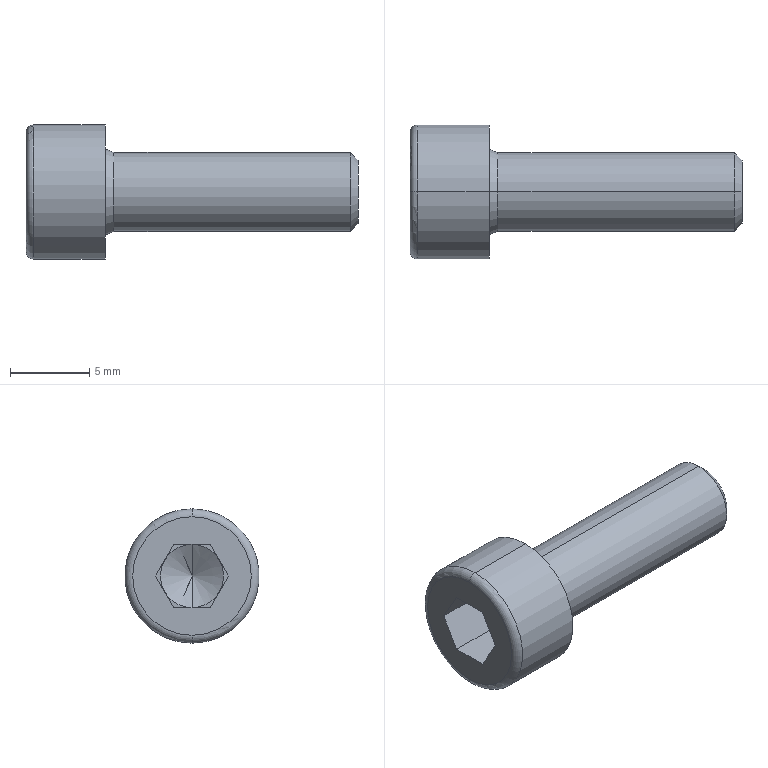Part | STEP file | 1 solid | 27 faces | box 21 x 8.5 x 8.5 mm | volume 547.894 mm3 | plane 15 | cone 6 | cylinder 4 | torus 2 | commonest cylinder face diameters 5 x2 8.5 x2
STEP:
#1=CARTESIAN_POINT('',(-0.7453,0.,0.));
#2=VERTEX_POINT('',#1);
#3=CARTESIAN_POINT('',(-1.9,0.,2.));
#4=VERTEX_POINT('',#3);
#5=CARTESIAN_POINT('',(-1.9,0.,2.));
#6=DIRECTION('',(-0.5,0.,0.866));
#7=VECTOR('',#6,1000.);
#8=LINE('',#5,#7);
#9=EDGE_CURVE('',#2,#4,#8,.T.);
#10=ORIENTED_EDGE('',*,*,#9,.F.);
#11=CARTESIAN_POINT('',(-1.9,0.,-2.));
#12=VERTEX_POINT('',#11);
#13=CARTESIAN_POINT('',(-1.9,0.,-2.));
#14=DIRECTION('',(-0.5,0.,-0.866));
#15=VECTOR('',#14,1000.);
#16=LINE('',#13,#15);
#17=EDGE_CURVE('',#2,#12,#16,.T.);
#18=ORIENTED_EDGE('',*,*,#17,.T.);
#19=CARTESIAN_POINT('',(-1.9,-1.732,-1.));
#20=VERTEX_POINT('',#19);
#21=CARTESIAN_POINT('',(-1.9,0.,0.));
#22=DIRECTION('',(-1.,0.,0.));
#23=DIRECTION('',(0.,0.,1.));
#24=AXIS2_PLACEMENT_3D('',#21,#22,#23);
#25=CIRCLE('',#24,2.);
#26=EDGE_CURVE('',#12,#20,#25,.T.);
#27=ORIENTED_EDGE('',*,*,#26,.T.);
#28=CARTESIAN_POINT('',(-1.9,-1.732,1.));
#29=VERTEX_POINT('',#28);
#30=CARTESIAN_POINT('',(-1.9,0.,0.));
#31=DIRECTION('',(-1.,0.,0.));
#32=DIRECTION('',(0.,0.,1.));
#33=AXIS2_PLACEMENT_3D('',#30,#31,#32);
#34=CIRCLE('',#33,2.);
#35=EDGE_CURVE('',#20,#29,#34,.T.);
#36=ORIENTED_EDGE('',*,*,#35,.T.);
#37=CARTESIAN_POINT('',(-1.9,0.,0.));
#38=DIRECTION('',(-1.,0.,0.));
#39=DIRECTION('',(0.,0.,1.));
#40=AXIS2_PLACEMENT_3D('',#37,#38,#39);
#41=CIRCLE('',#40,2.);
#42=EDGE_CURVE('',#29,#4,#41,.T.);
#43=ORIENTED_EDGE('',*,*,#42,.T.);
#44=EDGE_LOOP('',(#10,#18,#27,#36,#43));
#45=FACE_OUTER_BOUND('',#44,.T.);
#46=CARTESIAN_POINT('',(-1.9,0.,0.));
#47=DIRECTION('',(-1.,0.,0.));
#48=DIRECTION('',(0.,0.,1.));
#49=AXIS2_PLACEMENT_3D('',#46,#47,#48);
#50=CONICAL_SURFACE('',#49,2.,1.047);
#51=ADVANCED_FACE('',(#45),#50,.F.);
#52=CARTESIAN_POINT('',(16.,0.,2.01));
#53=VERTEX_POINT('',#52);
#54=CARTESIAN_POINT('',(16.,0.,-2.01));
#55=VERTEX_POINT('',#54);
#56=CARTESIAN_POINT('',(16.,0.,0.));
#57=DIRECTION('',(-1.,0.,0.));
#58=DIRECTION('',(0.,0.,1.));
#59=AXIS2_PLACEMENT_3D('',#56,#57,#58);
#60=CIRCLE('',#59,2.01);
#61=EDGE_CURVE('',#53,#55,#60,.T.);
#62=ORIENTED_EDGE('',*,*,#61,.T.);
#63=CARTESIAN_POINT('',(15.509,0.,-2.5));
#64=VERTEX_POINT('',#63);
#65=CARTESIAN_POINT('',(16.,0.,-2.01));
#66=DIRECTION('',(-0.7071,0.,-0.7071));
#67=VECTOR('',#66,1000.);
#68=LINE('',#65,#67);
#69=EDGE_CURVE('',#55,#64,#68,.T.);
#70=ORIENTED_EDGE('',*,*,#69,.T.);
#71=CARTESIAN_POINT('',(15.509,0.,2.5));
#72=VERTEX_POINT('',#71);
#73=CARTESIAN_POINT('',(15.509,0.,0.));
#74=DIRECTION('',(-1.,0.,0.));
#75=DIRECTION('',(0.,0.,1.));
#76=AXIS2_PLACEMENT_3D('',#73,#74,#75);
#77=CIRCLE('',#76,2.5);
#78=EDGE_CURVE('',#72,#64,#77,.T.);
#79=ORIENTED_EDGE('',*,*,#78,.F.);
#80=CARTESIAN_POINT('',(16.,0.,2.01));
#81=DIRECTION('',(-0.7071,0.,0.7071));
#82=VECTOR('',#81,1000.);
#83=LINE('',#80,#82);
#84=EDGE_CURVE('',#53,#72,#83,.T.);
#85=ORIENTED_EDGE('',*,*,#84,.F.);
#86=EDGE_LOOP('',(#62,#70,#79,#85));
#87=FACE_OUTER_BOUND('',#86,.T.);
#88=CARTESIAN_POINT('',(16.,0.,0.));
#89=DIRECTION('',(-1.,0.,0.));
#90=DIRECTION('',(0.,0.,1.));
#91=AXIS2_PLACEMENT_3D('',#88,#89,#90);
#92=CONICAL_SURFACE('',#91,2.01,0.7854);
#93=ADVANCED_FACE('',(#87),#92,.T.);
#94=ORIENTED_EDGE('',*,*,#78,.T.);
#95=CARTESIAN_POINT('',(0.5637,0.,-2.5));
#96=VERTEX_POINT('',#95);
#97=CARTESIAN_POINT('',(16.,0.,-2.5));
#98=DIRECTION('',(-1.,0.,0.));
#99=VECTOR('',#98,1000.);
#100=LINE('',#97,#99);
#101=EDGE_CURVE('',#64,#96,#100,.T.);
#102=ORIENTED_EDGE('',*,*,#101,.T.);
#103=CARTESIAN_POINT('',(0.5637,0.,2.5));
#104=VERTEX_POINT('',#103);
#105=CARTESIAN_POINT('',(0.5637,0.,0.));
#106=DIRECTION('',(-1.,0.,0.));
#107=DIRECTION('',(0.,0.,1.));
#108=AXIS2_PLACEMENT_3D('',#105,#106,#107);
#109=CIRCLE('',#108,2.5);
#110=EDGE_CURVE('',#104,#96,#109,.T.);
#111=ORIENTED_EDGE('',*,*,#110,.F.);
#112=CARTESIAN_POINT('',(16.,0.,2.5));
#113=DIRECTION('',(-1.,0.,0.));
#114=VECTOR('',#113,1000.);
#115=LINE('',#112,#114);
#116=EDGE_CURVE('',#72,#104,#115,.T.);
#117=ORIENTED_EDGE('',*,*,#116,.F.);
#118=EDGE_LOOP('',(#94,#102,#111,#117));
#119=FACE_OUTER_BOUND('',#118,.T.);
#120=CARTESIAN_POINT('',(16.,0.,0.));
#121=DIRECTION('',(-1.,0.,0.));
#122=DIRECTION('',(0.,0.,1.));
#123=AXIS2_PLACEMENT_3D('',#120,#121,#122);
#124=CYLINDRICAL_SURFACE('',#123,2.5);
#125=ADVANCED_FACE('',(#119),#124,.T.);
#126=ORIENTED_EDGE('',*,*,#110,.T.);
#127=CARTESIAN_POINT('',(0.,0.,-2.711));
#128=VERTEX_POINT('',#127);
#129=CARTESIAN_POINT('',(0.5637,0.,-2.5));
#130=DIRECTION('',(-0.9363,0.,-0.3511));
#131=VECTOR('',#130,1000.);
#132=LINE('',#129,#131);
#133=EDGE_CURVE('',#96,#128,#132,.T.);
#134=ORIENTED_EDGE('',*,*,#133,.T.);
#135=CARTESIAN_POINT('',(0.,0.,2.711));
#136=VERTEX_POINT('',#135);
#137=CARTESIAN_POINT('',(0.,0.,0.));
#138=DIRECTION('',(-1.,0.,0.));
#139=DIRECTION('',(0.,0.,1.));
#140=AXIS2_PLACEMENT_3D('',#137,#138,#139);
#141=CIRCLE('',#140,2.711);
#142=EDGE_CURVE('',#136,#128,#141,.T.);
#143=ORIENTED_EDGE('',*,*,#142,.F.);
#144=CARTESIAN_POINT('',(0.5637,0.,2.5));
#145=DIRECTION('',(-0.9363,0.,0.3511));
#146=VECTOR('',#145,1000.);
#147=LINE('',#144,#146);
#148=EDGE_CURVE('',#104,#136,#147,.T.);
#149=ORIENTED_EDGE('',*,*,#148,.F.);
#150=EDGE_LOOP('',(#126,#134,#143,#149));
#151=FACE_OUTER_BOUND('',#150,.T.);
#152=CARTESIAN_POINT('',(0.5637,0.,0.));
#153=DIRECTION('',(-1.,0.,0.));
#154=DIRECTION('',(0.,0.,1.));
#155=AXIS2_PLACEMENT_3D('',#152,#153,#154);
#156=CONICAL_SURFACE('',#155,2.5,0.3588);
#157=ADVANCED_FACE('',(#151),#156,.T.);
#158=CARTESIAN_POINT('',(0.,0.,4.25));
#159=VERTEX_POINT('',#158);
#160=CARTESIAN_POINT('',(0.,0.,-4.25));
#161=VERTEX_POINT('',#160);
#162=CARTESIAN_POINT('',(0.,0.,0.));
#163=DIRECTION('',(-1.,0.,0.));
#164=DIRECTION('',(0.,0.,1.));
#165=AXIS2_PLACEMENT_3D('',#162,#163,#164);
#166=CIRCLE('',#165,4.25);
#167=EDGE_CURVE('',#159,#161,#166,.T.);
#168=ORIENTED_EDGE('',*,*,#167,.T.);
#169=CARTESIAN_POINT('',(-4.5,0.,-4.25));
#170=VERTEX_POINT('',#169);
#171=CARTESIAN_POINT('',(16.,0.,-4.25));
#172=DIRECTION('',(-1.,0.,0.));
#173=VECTOR('',#172,1000.);
#174=LINE('',#171,#173);
#175=EDGE_CURVE('',#161,#170,#174,.T.);
#176=ORIENTED_EDGE('',*,*,#175,.T.);
#177=CARTESIAN_POINT('',(-4.5,0.,4.25));
#178=VERTEX_POINT('',#177);
#179=CARTESIAN_POINT('',(-4.5,0.,0.));
#180=DIRECTION('',(-1.,0.,0.));
#181=DIRECTION('',(0.,0.,1.));
#182=AXIS2_PLACEMENT_3D('',#179,#180,#181);
#183=CIRCLE('',#182,4.25);
#184=EDGE_CURVE('',#178,#170,#183,.T.);
#185=ORIENTED_EDGE('',*,*,#184,.F.);
#186=CARTESIAN_POINT('',(16.,0.,4.25));
#187=DIRECTION('',(-1.,0.,0.));
#188=VECTOR('',#187,1000.);
#189=LINE('',#186,#188);
#190=EDGE_CURVE('',#159,#178,#189,.T.);
#191=ORIENTED_EDGE('',*,*,#190,.F.);
#192=EDGE_LOOP('',(#168,#176,#185,#191));
#193=FACE_OUTER_BOUND('',#192,.T.);
#194=CARTESIAN_POINT('',(16.,0.,0.));
#195=DIRECTION('',(-1.,0.,0.));
#196=DIRECTION('',(0.,0.,1.));
#197=AXIS2_PLACEMENT_3D('',#194,#195,#196);
#198=CYLINDRICAL_SURFACE('',#197,4.25);
#199=ADVANCED_FACE('',(#193),#198,.T.);
#200=ORIENTED_EDGE('',*,*,#184,.T.);
#201=CARTESIAN_POINT('',(-5.,0.,-3.75));
#202=VERTEX_POINT('',#201);
#203=CARTESIAN_POINT('',(-4.5,0.,-3.75));
#204=DIRECTION('',(0.,1.,0.));
#205=DIRECTION('',(0.,0.,1.));
#206=AXIS2_PLACEMENT_3D('',#203,#204,#205);
#207=CIRCLE('',#206,0.5);
#208=EDGE_CURVE('',#170,#202,#207,.T.);
#209=ORIENTED_EDGE('',*,*,#208,.T.);
#210=CARTESIAN_POINT('',(-5.,0.,3.75));
#211=VERTEX_POINT('',#210);
#212=CARTESIAN_POINT('',(-5.,0.,0.));
#213=DIRECTION('',(-1.,0.,0.));
#214=DIRECTION('',(0.,0.,1.));
#215=AXIS2_PLACEMENT_3D('',#212,#213,#214);
#216=CIRCLE('',#215,3.75);
#217=EDGE_CURVE('',#211,#202,#216,.T.);
#218=ORIENTED_EDGE('',*,*,#217,.F.);
#219=CARTESIAN_POINT('',(-4.5,0.,3.75));
#220=DIRECTION('',(0.,-1.,0.));
#221=DIRECTION('',(0.,0.,-1.));
#222=AXIS2_PLACEMENT_3D('',#219,#220,#221);
#223=CIRCLE('',#222,0.5);
#224=EDGE_CURVE('',#178,#211,#223,.T.);
#225=ORIENTED_EDGE('',*,*,#224,.F.);
#226=EDGE_LOOP('',(#200,#209,#218,#225));
#227=FACE_OUTER_BOUND('',#226,.T.);
#228=CARTESIAN_POINT('',(-4.5,0.,0.));
#229=DIRECTION('',(-1.,0.,0.));
#230=DIRECTION('',(0.,0.,1.));
#231=AXIS2_PLACEMENT_3D('',#228,#229,#230);
#232=TOROIDAL_SURFACE('',#231,3.75,0.5);
#233=ADVANCED_FACE('',(#227),#232,.T.);
#234=CARTESIAN_POINT('',(-5.,-2.309,0.));
#235=VERTEX_POINT('',#234);
#236=CARTESIAN_POINT('',(-5.,-1.155,-2.));
#237=VERTEX_POINT('',#236);
#238=CARTESIAN_POINT('',(-5.,-1.232,-1.866));
#239=DIRECTION('',(0.,0.5,-0.866));
#240=VECTOR('',#239,1000.);
#241=LINE('',#238,#240);
#242=EDGE_CURVE('',#235,#237,#241,.T.);
#243=ORIENTED_EDGE('',*,*,#242,.T.);
#244=CARTESIAN_POINT('',(-5.,1.155,-2.));
#245=VERTEX_POINT('',#244);
#246=CARTESIAN_POINT('',(-5.,2.,-2.));
#247=DIRECTION('',(0.,1.,0.));
#248=VECTOR('',#247,1000.);
#249=LINE('',#246,#248);
#250=EDGE_CURVE('',#237,#245,#249,.T.);
#251=ORIENTED_EDGE('',*,*,#250,.T.);
#252=CARTESIAN_POINT('',(-5.,2.309,0.));
#253=VERTEX_POINT('',#252);
#254=CARTESIAN_POINT('',(-5.,2.232,-0.134));
#255=DIRECTION('',(0.,0.5,0.866));
#256=VECTOR('',#255,1000.);
#257=LINE('',#254,#256);
#258=EDGE_CURVE('',#245,#253,#257,.T.);
#259=ORIENTED_EDGE('',*,*,#258,.T.);
#260=CARTESIAN_POINT('',(-5.,1.155,2.));
#261=VERTEX_POINT('',#260);
#262=CARTESIAN_POINT('',(-5.,2.232,0.134));
#263=DIRECTION('',(0.,-0.5,0.866));
#264=VECTOR('',#263,1000.);
#265=LINE('',#262,#264);
#266=EDGE_CURVE('',#253,#261,#265,.T.);
#267=ORIENTED_EDGE('',*,*,#266,.T.);
#268=CARTESIAN_POINT('',(-5.,-1.155,2.));
#269=VERTEX_POINT('',#268);
#270=CARTESIAN_POINT('',(-5.,2.,2.));
#271=DIRECTION('',(0.,-1.,0.));
#272=VECTOR('',#271,1000.);
#273=LINE('',#270,#272);
#274=EDGE_CURVE('',#261,#269,#273,.T.);
#275=ORIENTED_EDGE('',*,*,#274,.T.);
#276=CARTESIAN_POINT('',(-5.,-1.232,1.866));
#277=DIRECTION('',(0.,-0.5,-0.866));
#278=VECTOR('',#277,1000.);
#279=LINE('',#276,#278);
#280=EDGE_CURVE('',#269,#235,#279,.T.);
#281=ORIENTED_EDGE('',*,*,#280,.T.);
#282=EDGE_LOOP('',(#243,#251,#259,#267,#275,#281));
#283=FACE_BOUND('',#282,.T.);
#284=ORIENTED_EDGE('',*,*,#217,.T.);
#285=CARTESIAN_POINT('',(-5.,0.,0.));
#286=DIRECTION('',(-1.,0.,0.));
#287=DIRECTION('',(0.,0.,1.));
#288=AXIS2_PLACEMENT_3D('',#285,#286,#287);
#289=CIRCLE('',#288,3.75);
#290=EDGE_CURVE('',#202,#211,#289,.T.);
#291=ORIENTED_EDGE('',*,*,#290,.T.);
#292=EDGE_LOOP('',(#284,#291));
#293=FACE_OUTER_BOUND('',#292,.T.);
#294=CARTESIAN_POINT('',(-5.,2.,0.));
#295=DIRECTION('',(1.,0.,0.));
#296=DIRECTION('',(0.,0.,-1.));
#297=AXIS2_PLACEMENT_3D('',#294,#295,#296);
#298=PLANE('',#297);
#299=ADVANCED_FACE('',(#283,#293),#298,.F.);
#300=ORIENTED_EDGE('',*,*,#208,.F.);
#301=CARTESIAN_POINT('',(-4.5,0.,0.));
#302=DIRECTION('',(-1.,0.,0.));
#303=DIRECTION('',(0.,0.,1.));
#304=AXIS2_PLACEMENT_3D('',#301,#302,#303);
#305=CIRCLE('',#304,4.25);
#306=EDGE_CURVE('',#170,#178,#305,.T.);
#307=ORIENTED_EDGE('',*,*,#306,.T.);
#308=ORIENTED_EDGE('',*,*,#224,.T.);
#309=ORIENTED_EDGE('',*,*,#290,.F.);
#310=EDGE_LOOP('',(#300,#307,#308,#309));
#311=FACE_OUTER_BOUND('',#310,.T.);
#312=CARTESIAN_POINT('',(-4.5,0.,0.));
#313=DIRECTION('',(-1.,0.,0.));
#314=DIRECTION('',(0.,0.,1.));
#315=AXIS2_PLACEMENT_3D('',#312,#313,#314);
#316=TOROIDAL_SURFACE('',#315,3.75,0.5);
#317=ADVANCED_FACE('',(#311),#316,.T.);
#318=ORIENTED_EDGE('',*,*,#175,.F.);
#319=CARTESIAN_POINT('',(0.,0.,0.));
#320=DIRECTION('',(-1.,0.,0.));
#321=DIRECTION('',(0.,0.,1.));
#322=AXIS2_PLACEMENT_3D('',#319,#320,#321);
#323=CIRCLE('',#322,4.25);
#324=EDGE_CURVE('',#161,#159,#323,.T.);
#325=ORIENTED_EDGE('',*,*,#324,.T.);
#326=ORIENTED_EDGE('',*,*,#190,.T.);
#327=ORIENTED_EDGE('',*,*,#306,.F.);
#328=EDGE_LOOP('',(#318,#325,#326,#327));
#329=FACE_OUTER_BOUND('',#328,.T.);
#330=CARTESIAN_POINT('',(16.,0.,0.));
#331=DIRECTION('',(-1.,0.,0.));
#332=DIRECTION('',(0.,0.,1.));
#333=AXIS2_PLACEMENT_3D('',#330,#331,#332);
#334=CYLINDRICAL_SURFACE('',#333,4.25);
#335=ADVANCED_FACE('',(#329),#334,.T.);
#336=ORIENTED_EDGE('',*,*,#167,.F.);
#337=ORIENTED_EDGE('',*,*,#324,.F.);
#338=EDGE_LOOP('',(#336,#337));
#339=FACE_OUTER_BOUND('',#338,.T.);
#340=ORIENTED_EDGE('',*,*,#142,.T.);
#341=CARTESIAN_POINT('',(0.,0.,0.));
#342=DIRECTION('',(-1.,0.,0.));
#343=DIRECTION('',(0.,0.,1.));
#344=AXIS2_PLACEMENT_3D('',#341,#342,#343);
#345=CIRCLE('',#344,2.711);
#346=EDGE_CURVE('',#128,#136,#345,.T.);
#347=ORIENTED_EDGE('',*,*,#346,.T.);
#348=EDGE_LOOP('',(#340,#347));
#349=FACE_BOUND('',#348,.T.);
#350=CARTESIAN_POINT('',(0.,4.25,0.));
#351=DIRECTION('',(-1.,0.,0.));
#352=DIRECTION('',(0.,0.,1.));
#353=AXIS2_PLACEMENT_3D('',#350,#351,#352);
#354=PLANE('',#353);
#355=ADVANCED_FACE('',(#339,#349),#354,.F.);
#356=ORIENTED_EDGE('',*,*,#133,.F.);
#357=CARTESIAN_POINT('',(0.5637,0.,0.));
#358=DIRECTION('',(-1.,0.,0.));
#359=DIRECTION('',(0.,0.,1.));
#360=AXIS2_PLACEMENT_3D('',#357,#358,#359);
#361=CIRCLE('',#360,2.5);
#362=EDGE_CURVE('',#96,#104,#361,.T.);
#363=ORIENTED_EDGE('',*,*,#362,.T.);
#364=ORIENTED_EDGE('',*,*,#148,.T.);
#365=ORIENTED_EDGE('',*,*,#346,.F.);
#366=EDGE_LOOP('',(#356,#363,#364,#365));
#367=FACE_OUTER_BOUND('',#366,.T.);
#368=CARTESIAN_POINT('',(0.5637,0.,0.));
#369=DIRECTION('',(-1.,0.,0.));
#370=DIRECTION('',(0.,0.,1.));
#371=AXIS2_PLACEMENT_3D('',#368,#369,#370);
#372=CONICAL_SURFACE('',#371,2.5,0.3588);
#373=ADVANCED_FACE('',(#367),#372,.T.);
#374=ORIENTED_EDGE('',*,*,#101,.F.);
#375=CARTESIAN_POINT('',(15.509,0.,0.));
#376=DIRECTION('',(-1.,0.,0.));
#377=DIRECTION('',(0.,0.,1.));
#378=AXIS2_PLACEMENT_3D('',#375,#376,#377);
#379=CIRCLE('',#378,2.5);
#380=EDGE_CURVE('',#64,#72,#379,.T.);
#381=ORIENTED_EDGE('',*,*,#380,.T.);
#382=ORIENTED_EDGE('',*,*,#116,.T.);
#383=ORIENTED_EDGE('',*,*,#362,.F.);
#384=EDGE_LOOP('',(#374,#381,#382,#383));
#385=FACE_OUTER_BOUND('',#384,.T.);
#386=CARTESIAN_POINT('',(16.,0.,0.));
#387=DIRECTION('',(-1.,0.,0.));
#388=DIRECTION('',(0.,0.,1.));
#389=AXIS2_PLACEMENT_3D('',#386,#387,#388);
#390=CYLINDRICAL_SURFACE('',#389,2.5);
#391=ADVANCED_FACE('',(#385),#390,.T.);
#392=ORIENTED_EDGE('',*,*,#69,.F.);
#393=CARTESIAN_POINT('',(16.,0.,0.));
#394=DIRECTION('',(-1.,0.,0.));
#395=DIRECTION('',(0.,0.,1.));
#396=AXIS2_PLACEMENT_3D('',#393,#394,#395);
#397=CIRCLE('',#396,2.01);
#398=EDGE_CURVE('',#55,#53,#397,.T.);
#399=ORIENTED_EDGE('',*,*,#398,.T.);
#400=ORIENTED_EDGE('',*,*,#84,.T.);
#401=ORIENTED_EDGE('',*,*,#380,.F.);
#402=EDGE_LOOP('',(#392,#399,#400,#401));
#403=FACE_OUTER_BOUND('',#402,.T.);
#404=CARTESIAN_POINT('',(16.,0.,0.));
#405=DIRECTION('',(-1.,0.,0.));
#406=DIRECTION('',(0.,0.,1.));
#407=AXIS2_PLACEMENT_3D('',#404,#405,#406);
#408=CONICAL_SURFACE('',#407,2.01,0.7854);
#409=ADVANCED_FACE('',(#403),#408,.T.);
#410=ORIENTED_EDGE('',*,*,#61,.F.);
#411=ORIENTED_EDGE('',*,*,#398,.F.);
#412=EDGE_LOOP('',(#410,#411));
#413=FACE_OUTER_BOUND('',#412,.T.);
#414=CARTESIAN_POINT('',(16.,2.01,0.));
#415=DIRECTION('',(-1.,0.,0.));
#416=DIRECTION('',(0.,0.,1.));
#417=AXIS2_PLACEMENT_3D('',#414,#415,#416);
#418=PLANE('',#417);
#419=ADVANCED_FACE('',(#413),#418,.F.);
#420=CARTESIAN_POINT('',(-1.9,-1.155,-2.));
#421=VERTEX_POINT('',#420);
#422=CARTESIAN_POINT('',(-1.9,-1.155,-2.));
#423=DIRECTION('',(0.,1.,0.));
#424=VECTOR('',#423,1000.);
#425=LINE('',#422,#424);
#426=EDGE_CURVE('',#421,#12,#425,.T.);
#427=ORIENTED_EDGE('',*,*,#426,.F.);
#428=CARTESIAN_POINT('',(-1.9,-2.309,0.));
#429=DIRECTION('',(0.,0.5,-0.866));
#430=VECTOR('',#429,1000.);
#431=LINE('',#428,#430);
#432=EDGE_CURVE('',#20,#421,#431,.T.);
#433=ORIENTED_EDGE('',*,*,#432,.F.);
#434=ORIENTED_EDGE('',*,*,#26,.F.);
#435=EDGE_LOOP('',(#427,#433,#434));
#436=FACE_OUTER_BOUND('',#435,.T.);
#437=CARTESIAN_POINT('',(-1.9,0.,0.));
#438=DIRECTION('',(1.,0.,0.));
#439=DIRECTION('',(0.,0.,-1.));
#440=AXIS2_PLACEMENT_3D('',#437,#438,#439);
#441=PLANE('',#440);
#442=ADVANCED_FACE('',(#436),#441,.F.);
#443=CARTESIAN_POINT('',(-1.9,-2.309,0.));
#444=VERTEX_POINT('',#443);
#445=CARTESIAN_POINT('',(-1.9,-2.309,0.));
#446=DIRECTION('',(0.,0.5,-0.866));
#447=VECTOR('',#446,1000.);
#448=LINE('',#445,#447);
#449=EDGE_CURVE('',#444,#20,#448,.T.);
#450=ORIENTED_EDGE('',*,*,#449,.F.);
#451=CARTESIAN_POINT('',(-1.9,-1.155,2.));
#452=DIRECTION('',(0.,-0.5,-0.866));
#453=VECTOR('',#452,1000.);
#454=LINE('',#451,#453);
#455=EDGE_CURVE('',#29,#444,#454,.T.);
#456=ORIENTED_EDGE('',*,*,#455,.F.);
#457=ORIENTED_EDGE('',*,*,#35,.F.);
#458=EDGE_LOOP('',(#450,#456,#457));
#459=FACE_OUTER_BOUND('',#458,.T.);
#460=CARTESIAN_POINT('',(-1.9,0.,0.));
#461=DIRECTION('',(1.,0.,0.));
#462=DIRECTION('',(0.,0.,-1.));
#463=AXIS2_PLACEMENT_3D('',#460,#461,#462);
#464=PLANE('',#463);
#465=ADVANCED_FACE('',(#459),#464,.F.);
#466=CARTESIAN_POINT('',(-1.9,-1.155,2.));
#467=VERTEX_POINT('',#466);
#468=CARTESIAN_POINT('',(-1.9,-1.155,2.));
#469=DIRECTION('',(0.,-0.5,-0.866));
#470=VECTOR('',#469,1000.);
#471=LINE('',#468,#470);
#472=EDGE_CURVE('',#467,#29,#471,.T.);
#473=ORIENTED_EDGE('',*,*,#472,.F.);
#474=CARTESIAN_POINT('',(-1.9,1.155,2.));
#475=DIRECTION('',(0.,-1.,0.));
#476=VECTOR('',#475,1000.);
#477=LINE('',#474,#476);
#478=EDGE_CURVE('',#4,#467,#477,.T.);
#479=ORIENTED_EDGE('',*,*,#478,.F.);
#480=ORIENTED_EDGE('',*,*,#42,.F.);
#481=EDGE_LOOP('',(#473,#479,#480));
#482=FACE_OUTER_BOUND('',#481,.T.);
#483=CARTESIAN_POINT('',(-1.9,0.,0.));
#484=DIRECTION('',(1.,0.,0.));
#485=DIRECTION('',(0.,0.,-1.));
#486=AXIS2_PLACEMENT_3D('',#483,#484,#485);
#487=PLANE('',#486);
#488=ADVANCED_FACE('',(#482),#487,.F.);
#489=CARTESIAN_POINT('',(-1.9,1.155,2.));
#490=VERTEX_POINT('',#489);
#491=CARTESIAN_POINT('',(-1.9,1.155,2.));
#492=DIRECTION('',(0.,-1.,0.));
#493=VECTOR('',#492,1000.);
#494=LINE('',#491,#493);
#495=EDGE_CURVE('',#490,#4,#494,.T.);
#496=ORIENTED_EDGE('',*,*,#495,.F.);
#497=CARTESIAN_POINT('',(-1.9,1.732,1.));
#498=VERTEX_POINT('',#497);
#499=CARTESIAN_POINT('',(-1.9,2.309,0.));
#500=DIRECTION('',(0.,-0.5,0.866));
#501=VECTOR('',#500,1000.);
#502=LINE('',#499,#501);
#503=EDGE_CURVE('',#498,#490,#502,.T.);
#504=ORIENTED_EDGE('',*,*,#503,.F.);
#505=CARTESIAN_POINT('',(-1.9,0.,0.));
#506=DIRECTION('',(-1.,0.,0.));
#507=DIRECTION('',(0.,0.,1.));
#508=AXIS2_PLACEMENT_3D('',#505,#506,#507);
#509=CIRCLE('',#508,2.);
#510=EDGE_CURVE('',#4,#498,#509,.T.);
#511=ORIENTED_EDGE('',*,*,#510,.F.);
#512=EDGE_LOOP('',(#496,#504,#511));
#513=FACE_OUTER_BOUND('',#512,.T.);
#514=CARTESIAN_POINT('',(-1.9,0.,0.));
#515=DIRECTION('',(1.,0.,0.));
#516=DIRECTION('',(0.,0.,-1.));
#517=AXIS2_PLACEMENT_3D('',#514,#515,#516);
#518=PLANE('',#517);
#519=ADVANCED_FACE('',(#513),#518,.F.);
#520=CARTESIAN_POINT('',(-1.9,2.309,0.));
#521=VERTEX_POINT('',#520);
#522=CARTESIAN_POINT('',(-1.9,2.309,0.));
#523=DIRECTION('',(0.,-0.5,0.866));
#524=VECTOR('',#523,1000.);
#525=LINE('',#522,#524);
#526=EDGE_CURVE('',#521,#498,#525,.T.);
#527=ORIENTED_EDGE('',*,*,#526,.F.);
#528=CARTESIAN_POINT('',(-1.9,1.732,-1.));
#529=VERTEX_POINT('',#528);
#530=CARTESIAN_POINT('',(-1.9,1.155,-2.));
#531=DIRECTION('',(0.,0.5,0.866));
#532=VECTOR('',#531,1000.);
#533=LINE('',#530,#532);
#534=EDGE_CURVE('',#529,#521,#533,.T.);
#535=ORIENTED_EDGE('',*,*,#534,.F.);
#536=CARTESIAN_POINT('',(-1.9,0.,0.));
#537=DIRECTION('',(-1.,0.,0.));
#538=DIRECTION('',(0.,0.,1.));
#539=AXIS2_PLACEMENT_3D('',#536,#537,#538);
#540=CIRCLE('',#539,2.);
#541=EDGE_CURVE('',#498,#529,#540,.T.);
#542=ORIENTED_EDGE('',*,*,#541,.F.);
#543=EDGE_LOOP('',(#527,#535,#542));
#544=FACE_OUTER_BOUND('',#543,.T.);
#545=CARTESIAN_POINT('',(-1.9,0.,0.));
#546=DIRECTION('',(1.,0.,0.));
#547=DIRECTION('',(0.,0.,-1.));
#548=AXIS2_PLACEMENT_3D('',#545,#546,#547);
#549=PLANE('',#548);
#550=ADVANCED_FACE('',(#544),#549,.F.);
#551=CARTESIAN_POINT('',(-1.9,1.155,-2.));
#552=VERTEX_POINT('',#551);
#553=CARTESIAN_POINT('',(-1.9,1.155,-2.));
#554=DIRECTION('',(0.,0.5,0.866));
#555=VECTOR('',#554,1000.);
#556=LINE('',#553,#555);
#557=EDGE_CURVE('',#552,#529,#556,.T.);
#558=ORIENTED_EDGE('',*,*,#557,.F.);
#559=CARTESIAN_POINT('',(-1.9,-1.155,-2.));
#560=DIRECTION('',(0.,1.,0.));
#561=VECTOR('',#560,1000.);
#562=LINE('',#559,#561);
#563=EDGE_CURVE('',#12,#552,#562,.T.);
#564=ORIENTED_EDGE('',*,*,#563,.F.);
#565=CARTESIAN_POINT('',(-1.9,0.,0.));
#566=DIRECTION('',(-1.,0.,0.));
#567=DIRECTION('',(0.,0.,1.));
#568=AXIS2_PLACEMENT_3D('',#565,#566,#567);
#569=CIRCLE('',#568,2.);
#570=EDGE_CURVE('',#529,#12,#569,.T.);
#571=ORIENTED_EDGE('',*,*,#570,.F.);
#572=EDGE_LOOP('',(#558,#564,#571));
#573=FACE_OUTER_BOUND('',#572,.T.);
#574=CARTESIAN_POINT('',(-1.9,0.,0.));
#575=DIRECTION('',(1.,0.,0.));
#576=DIRECTION('',(0.,0.,-1.));
#577=AXIS2_PLACEMENT_3D('',#574,#575,#576);
#578=PLANE('',#577);
#579=ADVANCED_FACE('',(#573),#578,.F.);
#580=ORIENTED_EDGE('',*,*,#266,.F.);
#581=CARTESIAN_POINT('',(-6.9,2.309,0.));
#582=DIRECTION('',(1.,0.,0.));
#583=VECTOR('',#582,1000.);
#584=LINE('',#581,#583);
#585=EDGE_CURVE('',#253,#521,#584,.T.);
#586=ORIENTED_EDGE('',*,*,#585,.T.);
#587=ORIENTED_EDGE('',*,*,#526,.T.);
#588=ORIENTED_EDGE('',*,*,#503,.T.);
#589=CARTESIAN_POINT('',(-6.9,1.155,2.));
#590=DIRECTION('',(1.,0.,0.));
#591=VECTOR('',#590,1000.);
#592=LINE('',#589,#591);
#593=EDGE_CURVE('',#261,#490,#592,.T.);
#594=ORIENTED_EDGE('',*,*,#593,.F.);
#595=EDGE_LOOP('',(#580,#586,#587,#588,#594));
#596=FACE_OUTER_BOUND('',#595,.T.);
#597=CARTESIAN_POINT('',(-6.9,2.309,0.));
#598=DIRECTION('',(0.,0.866,0.5));
#599=DIRECTION('',(0.,-0.5,0.866));
#600=AXIS2_PLACEMENT_3D('',#597,#598,#599);
#601=PLANE('',#600);
#602=ADVANCED_FACE('',(#596),#601,.F.);
#603=ORIENTED_EDGE('',*,*,#258,.F.);
#604=CARTESIAN_POINT('',(-6.9,1.155,-2.));
#605=DIRECTION('',(1.,0.,0.));
#606=VECTOR('',#605,1000.);
#607=LINE('',#604,#606);
#608=EDGE_CURVE('',#245,#552,#607,.T.);
#609=ORIENTED_EDGE('',*,*,#608,.T.);
#610=ORIENTED_EDGE('',*,*,#557,.T.);
#611=ORIENTED_EDGE('',*,*,#534,.T.);
#612=ORIENTED_EDGE('',*,*,#585,.F.);
#613=EDGE_LOOP('',(#603,#609,#610,#611,#612));
#614=FACE_OUTER_BOUND('',#613,.T.);
#615=CARTESIAN_POINT('',(-6.9,1.155,-2.));
#616=DIRECTION('',(0.,0.866,-0.5));
#617=DIRECTION('',(0.,0.5,0.866));
#618=AXIS2_PLACEMENT_3D('',#615,#616,#617);
#619=PLANE('',#618);
#620=ADVANCED_FACE('',(#614),#619,.F.);
#621=ORIENTED_EDGE('',*,*,#250,.F.);
#622=CARTESIAN_POINT('',(-6.9,-1.155,-2.));
#623=DIRECTION('',(1.,0.,0.));
#624=VECTOR('',#623,1000.);
#625=LINE('',#622,#624);
#626=EDGE_CURVE('',#237,#421,#625,.T.);
#627=ORIENTED_EDGE('',*,*,#626,.T.);
#628=ORIENTED_EDGE('',*,*,#426,.T.);
#629=ORIENTED_EDGE('',*,*,#563,.T.);
#630=ORIENTED_EDGE('',*,*,#608,.F.);
#631=EDGE_LOOP('',(#621,#627,#628,#629,#630));
#632=FACE_OUTER_BOUND('',#631,.T.);
#633=CARTESIAN_POINT('',(-6.9,-1.155,-2.));
#634=DIRECTION('',(0.,0.,-1.));
#635=DIRECTION('',(-1.,0.,0.));
#636=AXIS2_PLACEMENT_3D('',#633,#634,#635);
#637=PLANE('',#636);
#638=ADVANCED_FACE('',(#632),#637,.F.);
#639=ORIENTED_EDGE('',*,*,#242,.F.);
#640=CARTESIAN_POINT('',(-6.9,-2.309,0.));
#641=DIRECTION('',(1.,0.,0.));
#642=VECTOR('',#641,1000.);
#643=LINE('',#640,#642);
#644=EDGE_CURVE('',#235,#444,#643,.T.);
#645=ORIENTED_EDGE('',*,*,#644,.T.);
#646=ORIENTED_EDGE('',*,*,#449,.T.);
#647=ORIENTED_EDGE('',*,*,#432,.T.);
#648=ORIENTED_EDGE('',*,*,#626,.F.);
#649=EDGE_LOOP('',(#639,#645,#646,#647,#648));
#650=FACE_OUTER_BOUND('',#649,.T.);
#651=CARTESIAN_POINT('',(-6.9,-2.309,0.));
#652=DIRECTION('',(0.,-0.866,-0.5));
#653=DIRECTION('',(0.,0.5,-0.866));
#654=AXIS2_PLACEMENT_3D('',#651,#652,#653);
#655=PLANE('',#654);
#656=ADVANCED_FACE('',(#650),#655,.F.);
#657=ORIENTED_EDGE('',*,*,#280,.F.);
#658=CARTESIAN_POINT('',(-6.9,-1.155,2.));
#659=DIRECTION('',(1.,0.,0.));
#660=VECTOR('',#659,1000.);
#661=LINE('',#658,#660);
#662=EDGE_CURVE('',#269,#467,#661,.T.);
#663=ORIENTED_EDGE('',*,*,#662,.T.);
#664=ORIENTED_EDGE('',*,*,#472,.T.);
#665=ORIENTED_EDGE('',*,*,#455,.T.);
#666=ORIENTED_EDGE('',*,*,#644,.F.);
#667=EDGE_LOOP('',(#657,#663,#664,#665,#666));
#668=FACE_OUTER_BOUND('',#667,.T.);
#669=CARTESIAN_POINT('',(-6.9,-1.155,2.));
#670=DIRECTION('',(0.,-0.866,0.5));
#671=DIRECTION('',(0.,-0.5,-0.866));
#672=AXIS2_PLACEMENT_3D('',#669,#670,#671);
#673=PLANE('',#672);
#674=ADVANCED_FACE('',(#668),#673,.F.);
#675=ORIENTED_EDGE('',*,*,#274,.F.);
#676=ORIENTED_EDGE('',*,*,#593,.T.);
#677=ORIENTED_EDGE('',*,*,#495,.T.);
#678=ORIENTED_EDGE('',*,*,#478,.T.);
#679=ORIENTED_EDGE('',*,*,#662,.F.);
#680=EDGE_LOOP('',(#675,#676,#677,#678,#679));
#681=FACE_OUTER_BOUND('',#680,.T.);
#682=CARTESIAN_POINT('',(-6.9,1.155,2.));
#683=DIRECTION('',(0.,0.,1.));
#684=DIRECTION('',(1.,0.,0.));
#685=AXIS2_PLACEMENT_3D('',#682,#683,#684);
#686=PLANE('',#685);
#687=ADVANCED_FACE('',(#681),#686,.F.);
#688=ORIENTED_EDGE('',*,*,#17,.F.);
#689=ORIENTED_EDGE('',*,*,#9,.T.);
#690=ORIENTED_EDGE('',*,*,#510,.T.);
#691=ORIENTED_EDGE('',*,*,#541,.T.);
#692=ORIENTED_EDGE('',*,*,#570,.T.);
#693=EDGE_LOOP('',(#688,#689,#690,#691,#692));
#694=FACE_OUTER_BOUND('',#693,.T.);
#695=CARTESIAN_POINT('',(-1.9,0.,0.));
#696=DIRECTION('',(-1.,0.,0.));
#697=DIRECTION('',(0.,0.,1.));
#698=AXIS2_PLACEMENT_3D('',#695,#696,#697);
#699=CONICAL_SURFACE('',#698,2.,1.047);
#700=ADVANCED_FACE('',(#694),#699,.F.);
#701=CLOSED_SHELL('',(#51,#93,#125,#157,#199,#233,#299,#317,#335,#355,#373,#391,#409,#419,#442,#465,#488,#519,#550,#579,#602,#620,#638,#656,#674,#687,#700));
#702=MANIFOLD_SOLID_BREP('',#701);
#703=CARTESIAN_POINT('',(0.,0.,0.));
#704=DIRECTION('',(0.,0.,1.));
#705=DIRECTION('',(1.,0.,0.));
#706=AXIS2_PLACEMENT_3D('',#703,#704,#705);
#707=(LENGTH_UNIT()NAMED_UNIT(*)SI_UNIT(.MILLI.,.METRE.));
#708=UNCERTAINTY_MEASURE_WITH_UNIT(LENGTH_MEASURE(0.00001),#707,'','');
#709=(NAMED_UNIT(*)PLANE_ANGLE_UNIT()SI_UNIT($,.RADIAN.));
#710=(NAMED_UNIT(*)SI_UNIT($,.STERADIAN.)SOLID_ANGLE_UNIT());
#711=(GEOMETRIC_REPRESENTATION_CONTEXT(3)GLOBAL_UNCERTAINTY_ASSIGNED_CONTEXT((#708))GLOBAL_UNIT_ASSIGNED_CONTEXT((#707,#709,#710))REPRESENTATION_CONTEXT('',''));
#712=ADVANCED_BREP_SHAPE_REPRESENTATION('',(#702,#706),#711);